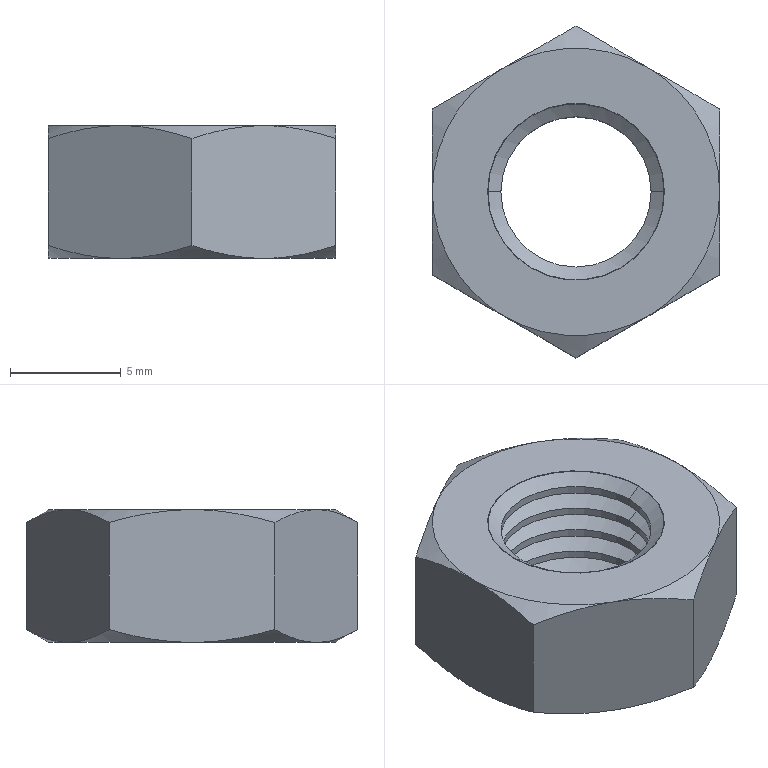Part | STEP file | Hex nut M8 | 1 solid | 56 faces | box 13 x 15.011 x 6 mm | volume 626.264 mm3 | cone 36 | cylinder 12 | plane 8 | commonest cylinder face diameters 6.8 x10 8 x2